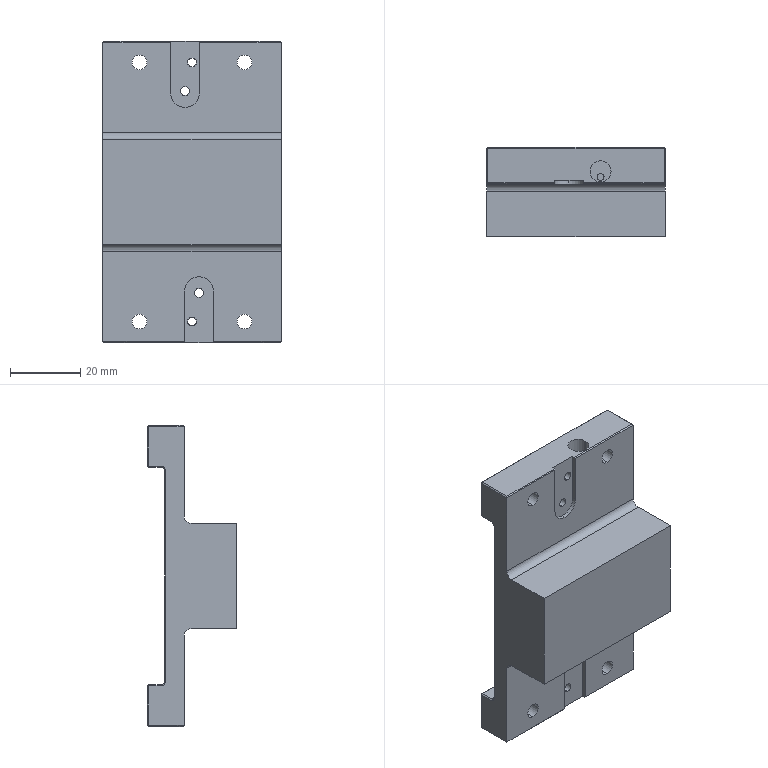Part | SolidWorks | features BaseBody 1 | 1 solid | 97 faces | box 51 x 25.5 x 86 mm | volume 51756 mm3 | plane 54 | cylinder 35 | cone 8 | commonest cylinder face diameters 2.5 x8 4.2 x8 2 x6 3 x4 6 x4 8.2 x3